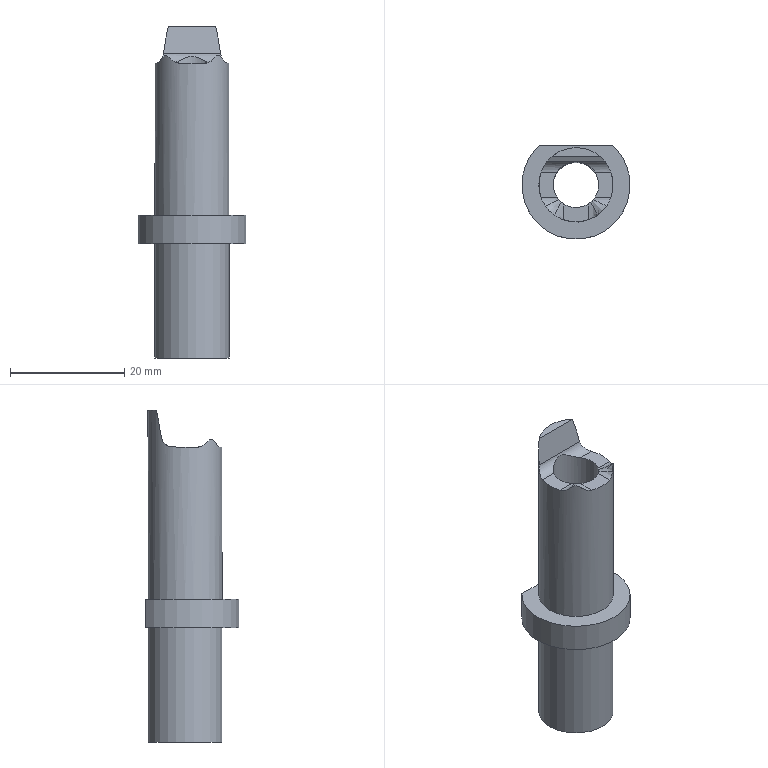Part | STEP file | P011002M014-000 | 1 solid | 20 faces | box 19 x 16.5 x 58.198 mm | volume 5006 mm3 | plane 8 | cylinder 7 | spline 4 | other 1 | commonest cylinder face diameters 4 x3 13 x2 8 x1 19 x1